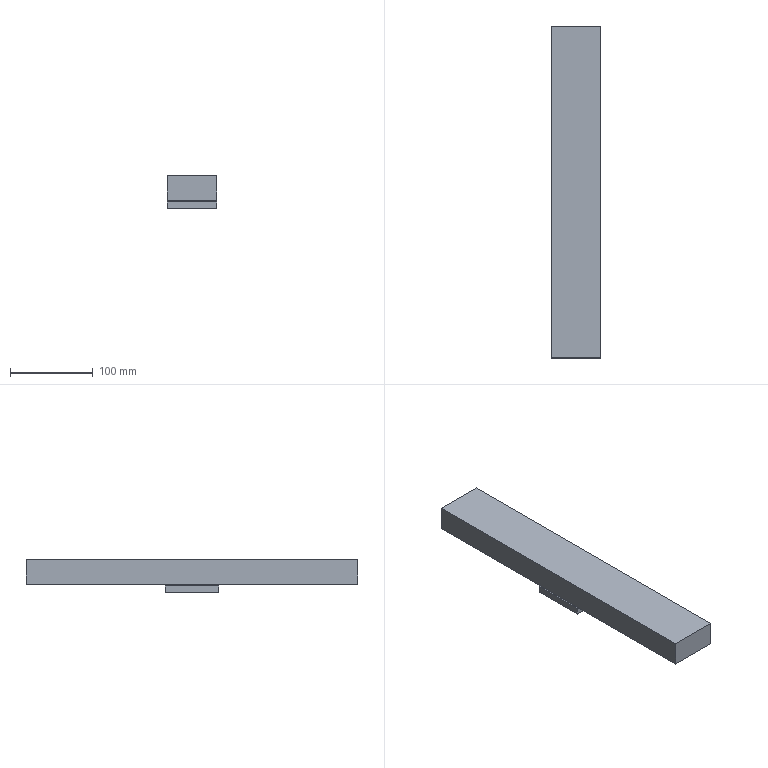Part | SolidWorks | features Cut 2, ICE 2, Chamfer 1, Extrusion 1, HoleWzd 1 | 1 solid | 13 faces | box 60 x 400 x 40 mm | volume 758635 mm3 | plane 13
STEP:
#1=CARTESIAN_POINT('',(-60.,32.5,8.));
#2=VERTEX_POINT('',#1);
#3=CARTESIAN_POINT('',(0.,32.5,8.));
#4=VERTEX_POINT('',#3);
#5=CARTESIAN_POINT('',(60.,32.5,8.));
#6=DIRECTION('',(1.,0.,0.));
#7=VECTOR('',#6,1000.);
#8=LINE('',#5,#7);
#9=EDGE_CURVE('',#2,#4,#8,.T.);
#10=ORIENTED_EDGE('',*,*,#9,.T.);
#11=CARTESIAN_POINT('',(0.,32.5,0.));
#12=VERTEX_POINT('',#11);
#13=CARTESIAN_POINT('',(0.,32.5,-88.459));
#14=DIRECTION('',(0.,0.,1.));
#15=VECTOR('',#14,1000.);
#16=LINE('',#13,#15);
#17=EDGE_CURVE('',#12,#4,#16,.T.);
#18=ORIENTED_EDGE('',*,*,#17,.F.);
#19=CARTESIAN_POINT('',(-60.,32.5,0.));
#20=VERTEX_POINT('',#19);
#21=CARTESIAN_POINT('',(-60.,32.5,0.));
#22=DIRECTION('',(-1.,0.,0.));
#23=VECTOR('',#22,1000.);
#24=LINE('',#21,#23);
#25=EDGE_CURVE('',#12,#20,#24,.T.);
#26=ORIENTED_EDGE('',*,*,#25,.T.);
#27=CARTESIAN_POINT('',(-60.,32.5,10.));
#28=DIRECTION('',(0.,0.,-1.));
#29=VECTOR('',#28,1000.);
#30=LINE('',#27,#29);
#31=EDGE_CURVE('',#2,#20,#30,.T.);
#32=ORIENTED_EDGE('',*,*,#31,.F.);
#33=EDGE_LOOP('',(#10,#18,#26,#32));
#34=FACE_OUTER_BOUND('',#33,.T.);
#35=CARTESIAN_POINT('',(-60.,32.5,10.));
#36=DIRECTION('',(0.,-1.,0.));
#37=DIRECTION('',(0.,0.,-1.));
#38=AXIS2_PLACEMENT_3D('',#35,#36,#37);
#39=PLANE('',#38);
#40=ADVANCED_FACE('',(#34),#39,.F.);
#41=CARTESIAN_POINT('',(-60.,-32.5,8.));
#42=VERTEX_POINT('',#41);
#43=CARTESIAN_POINT('',(-60.,-32.5,0.));
#44=VERTEX_POINT('',#43);
#45=CARTESIAN_POINT('',(-60.,-32.5,10.));
#46=DIRECTION('',(0.,0.,-1.));
#47=VECTOR('',#46,1000.);
#48=LINE('',#45,#47);
#49=EDGE_CURVE('',#42,#44,#48,.T.);
#50=ORIENTED_EDGE('',*,*,#49,.F.);
#51=CARTESIAN_POINT('',(-60.,32.5,8.));
#52=DIRECTION('',(0.,1.,0.));
#53=VECTOR('',#52,1000.);
#54=LINE('',#51,#53);
#55=EDGE_CURVE('',#42,#2,#54,.T.);
#56=ORIENTED_EDGE('',*,*,#55,.T.);
#57=ORIENTED_EDGE('',*,*,#31,.T.);
#58=CARTESIAN_POINT('',(-60.,32.5,0.));
#59=DIRECTION('',(0.,-1.,0.));
#60=VECTOR('',#59,1000.);
#61=LINE('',#58,#60);
#62=EDGE_CURVE('',#20,#44,#61,.T.);
#63=ORIENTED_EDGE('',*,*,#62,.T.);
#64=EDGE_LOOP('',(#50,#56,#57,#63));
#65=FACE_OUTER_BOUND('',#64,.T.);
#66=CARTESIAN_POINT('',(-60.,32.5,10.));
#67=DIRECTION('',(1.,0.,0.));
#68=DIRECTION('',(0.,1.,0.));
#69=AXIS2_PLACEMENT_3D('',#66,#67,#68);
#70=PLANE('',#69);
#71=ADVANCED_FACE('',(#65),#70,.F.);
#72=CARTESIAN_POINT('',(0.,-32.5,0.));
#73=VERTEX_POINT('',#72);
#74=CARTESIAN_POINT('',(-60.,-32.5,0.));
#75=DIRECTION('',(1.,0.,0.));
#76=VECTOR('',#75,1000.);
#77=LINE('',#74,#76);
#78=EDGE_CURVE('',#44,#73,#77,.T.);
#79=ORIENTED_EDGE('',*,*,#78,.T.);
#80=CARTESIAN_POINT('',(0.,-32.5,8.));
#81=VERTEX_POINT('',#80);
#82=CARTESIAN_POINT('',(0.,-32.5,-88.459));
#83=DIRECTION('',(0.,0.,1.));
#84=VECTOR('',#83,1000.);
#85=LINE('',#82,#84);
#86=EDGE_CURVE('',#73,#81,#85,.T.);
#87=ORIENTED_EDGE('',*,*,#86,.T.);
#88=CARTESIAN_POINT('',(-60.,-32.5,8.));
#89=DIRECTION('',(-1.,0.,0.));
#90=VECTOR('',#89,1000.);
#91=LINE('',#88,#90);
#92=EDGE_CURVE('',#81,#42,#91,.T.);
#93=ORIENTED_EDGE('',*,*,#92,.T.);
#94=ORIENTED_EDGE('',*,*,#49,.T.);
#95=EDGE_LOOP('',(#79,#87,#93,#94));
#96=FACE_OUTER_BOUND('',#95,.T.);
#97=CARTESIAN_POINT('',(-60.,-32.5,10.));
#98=DIRECTION('',(0.,1.,0.));
#99=DIRECTION('',(0.,0.,1.));
#100=AXIS2_PLACEMENT_3D('',#97,#98,#99);
#101=PLANE('',#100);
#102=ADVANCED_FACE('',(#96),#101,.F.);
#103=ORIENTED_EDGE('',*,*,#25,.F.);
#104=CARTESIAN_POINT('',(0.,32.5,0.));
#105=DIRECTION('',(0.,1.,0.));
#106=VECTOR('',#105,1000.);
#107=LINE('',#104,#106);
#108=EDGE_CURVE('',#73,#12,#107,.T.);
#109=ORIENTED_EDGE('',*,*,#108,.F.);
#110=ORIENTED_EDGE('',*,*,#78,.F.);
#111=ORIENTED_EDGE('',*,*,#62,.F.);
#112=EDGE_LOOP('',(#103,#109,#110,#111));
#113=FACE_OUTER_BOUND('',#112,.T.);
#114=CARTESIAN_POINT('',(0.,0.,0.));
#115=DIRECTION('',(0.,0.,1.));
#116=DIRECTION('',(1.,0.,0.));
#117=AXIS2_PLACEMENT_3D('',#114,#115,#116);
#118=PLANE('',#117);
#119=ADVANCED_FACE('',(#113),#118,.F.);
#120=CARTESIAN_POINT('',(-58.,30.5,10.));
#121=VERTEX_POINT('',#120);
#122=CARTESIAN_POINT('',(-38.667,11.167,29.333));
#123=DIRECTION('',(0.5774,-0.5774,0.5774));
#124=VECTOR('',#123,1000.);
#125=LINE('',#122,#124);
#126=EDGE_CURVE('',#2,#121,#125,.T.);
#127=ORIENTED_EDGE('',*,*,#126,.F.);
#128=ORIENTED_EDGE('',*,*,#55,.F.);
#129=CARTESIAN_POINT('',(-58.,-30.5,10.));
#130=VERTEX_POINT('',#129);
#131=CARTESIAN_POINT('',(-47.833,-20.333,20.167));
#132=DIRECTION('',(-0.5774,-0.5774,-0.5774));
#133=VECTOR('',#132,1000.);
#134=LINE('',#131,#133);
#135=EDGE_CURVE('',#130,#42,#134,.T.);
#136=ORIENTED_EDGE('',*,*,#135,.F.);
#137=CARTESIAN_POINT('',(-58.,-32.5,10.));
#138=DIRECTION('',(0.,-1.,0.));
#139=VECTOR('',#138,1000.);
#140=LINE('',#137,#139);
#141=EDGE_CURVE('',#121,#130,#140,.T.);
#142=ORIENTED_EDGE('',*,*,#141,.F.);
#143=EDGE_LOOP('',(#127,#128,#136,#142));
#144=FACE_OUTER_BOUND('',#143,.T.);
#145=CARTESIAN_POINT('',(-58.,0.,10.));
#146=DIRECTION('',(-0.7071,0.,0.7071));
#147=DIRECTION('',(0.,1.,0.));
#148=AXIS2_PLACEMENT_3D('',#145,#146,#147);
#149=PLANE('',#148);
#150=ADVANCED_FACE('',(#144),#149,.T.);
#151=CARTESIAN_POINT('',(0.,-30.5,10.));
#152=VERTEX_POINT('',#151);
#153=CARTESIAN_POINT('',(0.,-30.5,10.));
#154=DIRECTION('',(0.,-0.7071,-0.7071));
#155=VECTOR('',#154,1000.);
#156=LINE('',#153,#155);
#157=EDGE_CURVE('',#152,#81,#156,.T.);
#158=ORIENTED_EDGE('',*,*,#157,.F.);
#159=CARTESIAN_POINT('',(60.,-30.5,10.));
#160=DIRECTION('',(1.,0.,0.));
#161=VECTOR('',#160,1000.);
#162=LINE('',#159,#161);
#163=EDGE_CURVE('',#130,#152,#162,.T.);
#164=ORIENTED_EDGE('',*,*,#163,.F.);
#165=ORIENTED_EDGE('',*,*,#135,.T.);
#166=ORIENTED_EDGE('',*,*,#92,.F.);
#167=EDGE_LOOP('',(#158,#164,#165,#166));
#168=FACE_OUTER_BOUND('',#167,.T.);
#169=CARTESIAN_POINT('',(0.,-30.5,10.));
#170=DIRECTION('',(0.,-0.7071,0.7071));
#171=DIRECTION('',(-1.,0.,0.));
#172=AXIS2_PLACEMENT_3D('',#169,#170,#171);
#173=PLANE('',#172);
#174=ADVANCED_FACE('',(#168),#173,.T.);
#175=CARTESIAN_POINT('',(0.,30.5,10.));
#176=VERTEX_POINT('',#175);
#177=CARTESIAN_POINT('',(0.,30.5,10.));
#178=DIRECTION('',(0.,-0.7071,0.7071));
#179=VECTOR('',#178,1000.);
#180=LINE('',#177,#179);
#181=EDGE_CURVE('',#4,#176,#180,.T.);
#182=ORIENTED_EDGE('',*,*,#181,.F.);
#183=ORIENTED_EDGE('',*,*,#9,.F.);
#184=ORIENTED_EDGE('',*,*,#126,.T.);
#185=CARTESIAN_POINT('',(-60.,30.5,10.));
#186=DIRECTION('',(-1.,0.,0.));
#187=VECTOR('',#186,1000.);
#188=LINE('',#185,#187);
#189=EDGE_CURVE('',#176,#121,#188,.T.);
#190=ORIENTED_EDGE('',*,*,#189,.F.);
#191=EDGE_LOOP('',(#182,#183,#184,#190));
#192=FACE_OUTER_BOUND('',#191,.T.);
#193=CARTESIAN_POINT('',(0.,30.5,10.));
#194=DIRECTION('',(0.,0.7071,0.7071));
#195=DIRECTION('',(1.,0.,0.));
#196=AXIS2_PLACEMENT_3D('',#193,#194,#195);
#197=PLANE('',#196);
#198=ADVANCED_FACE('',(#192),#197,.T.);
#199=CARTESIAN_POINT('',(0.,200.,10.));
#200=VERTEX_POINT('',#199);
#201=CARTESIAN_POINT('',(0.,200.,10.));
#202=DIRECTION('',(0.,-1.,0.));
#203=VECTOR('',#202,1000.);
#204=LINE('',#201,#203);
#205=EDGE_CURVE('',#200,#176,#204,.T.);
#206=ORIENTED_EDGE('',*,*,#205,.T.);
#207=ORIENTED_EDGE('',*,*,#189,.T.);
#208=ORIENTED_EDGE('',*,*,#141,.T.);
#209=ORIENTED_EDGE('',*,*,#163,.T.);
#210=CARTESIAN_POINT('',(0.,-200.,10.));
#211=VERTEX_POINT('',#210);
#212=CARTESIAN_POINT('',(0.,200.,10.));
#213=DIRECTION('',(0.,-1.,0.));
#214=VECTOR('',#213,1000.);
#215=LINE('',#212,#214);
#216=EDGE_CURVE('',#152,#211,#215,.T.);
#217=ORIENTED_EDGE('',*,*,#216,.T.);
#218=CARTESIAN_POINT('',(-60.,-200.,10.));
#219=VERTEX_POINT('',#218);
#220=CARTESIAN_POINT('',(0.,-200.,10.));
#221=DIRECTION('',(-1.,0.,0.));
#222=VECTOR('',#221,1000.);
#223=LINE('',#220,#222);
#224=EDGE_CURVE('',#211,#219,#223,.T.);
#225=ORIENTED_EDGE('',*,*,#224,.T.);
#226=CARTESIAN_POINT('',(-60.,200.,10.));
#227=VERTEX_POINT('',#226);
#228=CARTESIAN_POINT('',(-60.,32.5,10.));
#229=DIRECTION('',(0.,-1.,0.));
#230=VECTOR('',#229,1000.);
#231=LINE('',#228,#230);
#232=EDGE_CURVE('',#227,#219,#231,.T.);
#233=ORIENTED_EDGE('',*,*,#232,.F.);
#234=CARTESIAN_POINT('',(0.,200.,10.));
#235=DIRECTION('',(1.,0.,0.));
#236=VECTOR('',#235,1000.);
#237=LINE('',#234,#236);
#238=EDGE_CURVE('',#227,#200,#237,.T.);
#239=ORIENTED_EDGE('',*,*,#238,.T.);
#240=EDGE_LOOP('',(#206,#207,#208,#209,#217,#225,#233,#239));
#241=FACE_OUTER_BOUND('',#240,.T.);
#242=CARTESIAN_POINT('',(0.,0.,10.));
#243=DIRECTION('',(0.,0.,1.));
#244=DIRECTION('',(1.,0.,0.));
#245=AXIS2_PLACEMENT_3D('',#242,#243,#244);
#246=PLANE('',#245);
#247=ADVANCED_FACE('',(#241),#246,.F.);
#248=ORIENTED_EDGE('',*,*,#232,.T.);
#249=CARTESIAN_POINT('',(-60.,-200.,40.));
#250=VERTEX_POINT('',#249);
#251=CARTESIAN_POINT('',(-60.,-200.,-394.475));
#252=DIRECTION('',(0.,0.,1.));
#253=VECTOR('',#252,1000.);
#254=LINE('',#251,#253);
#255=EDGE_CURVE('',#219,#250,#254,.T.);
#256=ORIENTED_EDGE('',*,*,#255,.T.);
#257=CARTESIAN_POINT('',(-60.,200.,40.));
#258=VERTEX_POINT('',#257);
#259=CARTESIAN_POINT('',(-60.,32.5,40.));
#260=DIRECTION('',(0.,-1.,0.));
#261=VECTOR('',#260,1000.);
#262=LINE('',#259,#261);
#263=EDGE_CURVE('',#258,#250,#262,.T.);
#264=ORIENTED_EDGE('',*,*,#263,.F.);
#265=CARTESIAN_POINT('',(-60.,200.,-394.475));
#266=DIRECTION('',(0.,0.,1.));
#267=VECTOR('',#266,1000.);
#268=LINE('',#265,#267);
#269=EDGE_CURVE('',#227,#258,#268,.T.);
#270=ORIENTED_EDGE('',*,*,#269,.F.);
#271=EDGE_LOOP('',(#248,#256,#264,#270));
#272=FACE_OUTER_BOUND('',#271,.T.);
#273=CARTESIAN_POINT('',(-60.,32.5,40.));
#274=DIRECTION('',(1.,0.,0.));
#275=DIRECTION('',(0.,0.,-1.));
#276=AXIS2_PLACEMENT_3D('',#273,#274,#275);
#277=PLANE('',#276);
#278=ADVANCED_FACE('',(#272),#277,.F.);
#279=CARTESIAN_POINT('',(0.,-200.,40.));
#280=VERTEX_POINT('',#279);
#281=CARTESIAN_POINT('',(0.,-200.,40.));
#282=DIRECTION('',(1.,0.,0.));
#283=VECTOR('',#282,1000.);
#284=LINE('',#281,#283);
#285=EDGE_CURVE('',#250,#280,#284,.T.);
#286=ORIENTED_EDGE('',*,*,#285,.T.);
#287=CARTESIAN_POINT('',(0.,200.,40.));
#288=VERTEX_POINT('',#287);
#289=CARTESIAN_POINT('',(0.,200.,40.));
#290=DIRECTION('',(0.,1.,0.));
#291=VECTOR('',#290,1000.);
#292=LINE('',#289,#291);
#293=EDGE_CURVE('',#280,#288,#292,.T.);
#294=ORIENTED_EDGE('',*,*,#293,.T.);
#295=CARTESIAN_POINT('',(0.,200.,40.));
#296=DIRECTION('',(-1.,0.,0.));
#297=VECTOR('',#296,1000.);
#298=LINE('',#295,#297);
#299=EDGE_CURVE('',#288,#258,#298,.T.);
#300=ORIENTED_EDGE('',*,*,#299,.T.);
#301=ORIENTED_EDGE('',*,*,#263,.T.);
#302=EDGE_LOOP('',(#286,#294,#300,#301));
#303=FACE_OUTER_BOUND('',#302,.T.);
#304=CARTESIAN_POINT('',(0.,0.,40.));
#305=DIRECTION('',(0.,0.,1.));
#306=DIRECTION('',(1.,0.,0.));
#307=AXIS2_PLACEMENT_3D('',#304,#305,#306);
#308=PLANE('',#307);
#309=ADVANCED_FACE('',(#303),#308,.T.);
#310=ORIENTED_EDGE('',*,*,#224,.F.);
#311=CARTESIAN_POINT('',(0.,-200.,-394.475));
#312=DIRECTION('',(0.,0.,1.));
#313=VECTOR('',#312,1000.);
#314=LINE('',#311,#313);
#315=EDGE_CURVE('',#211,#280,#314,.T.);
#316=ORIENTED_EDGE('',*,*,#315,.T.);
#317=ORIENTED_EDGE('',*,*,#285,.F.);
#318=ORIENTED_EDGE('',*,*,#255,.F.);
#319=EDGE_LOOP('',(#310,#316,#317,#318));
#320=FACE_OUTER_BOUND('',#319,.T.);
#321=CARTESIAN_POINT('',(0.,-200.,-394.475));
#322=DIRECTION('',(0.,-1.,0.));
#323=DIRECTION('',(0.,0.,-1.));
#324=AXIS2_PLACEMENT_3D('',#321,#322,#323);
#325=PLANE('',#324);
#326=ADVANCED_FACE('',(#320),#325,.T.);
#327=ORIENTED_EDGE('',*,*,#293,.F.);
#328=ORIENTED_EDGE('',*,*,#315,.F.);
#329=ORIENTED_EDGE('',*,*,#216,.F.);
#330=ORIENTED_EDGE('',*,*,#157,.T.);
#331=ORIENTED_EDGE('',*,*,#86,.F.);
#332=ORIENTED_EDGE('',*,*,#108,.T.);
#333=ORIENTED_EDGE('',*,*,#17,.T.);
#334=ORIENTED_EDGE('',*,*,#181,.T.);
#335=ORIENTED_EDGE('',*,*,#205,.F.);
#336=CARTESIAN_POINT('',(0.,200.,-394.475));
#337=DIRECTION('',(0.,0.,1.));
#338=VECTOR('',#337,1000.);
#339=LINE('',#336,#338);
#340=EDGE_CURVE('',#200,#288,#339,.T.);
#341=ORIENTED_EDGE('',*,*,#340,.T.);
#342=EDGE_LOOP('',(#327,#328,#329,#330,#331,#332,#333,#334,#335,#341));
#343=FACE_OUTER_BOUND('',#342,.T.);
#344=CARTESIAN_POINT('',(0.,200.,-394.475));
#345=DIRECTION('',(1.,0.,0.));
#346=DIRECTION('',(0.,1.,0.));
#347=AXIS2_PLACEMENT_3D('',#344,#345,#346);
#348=PLANE('',#347);
#349=ADVANCED_FACE('',(#343),#348,.T.);
#350=ORIENTED_EDGE('',*,*,#238,.F.);
#351=ORIENTED_EDGE('',*,*,#269,.T.);
#352=ORIENTED_EDGE('',*,*,#299,.F.);
#353=ORIENTED_EDGE('',*,*,#340,.F.);
#354=EDGE_LOOP('',(#350,#351,#352,#353));
#355=FACE_OUTER_BOUND('',#354,.T.);
#356=CARTESIAN_POINT('',(0.,200.,-394.475));
#357=DIRECTION('',(0.,1.,0.));
#358=DIRECTION('',(0.,0.,1.));
#359=AXIS2_PLACEMENT_3D('',#356,#357,#358);
#360=PLANE('',#359);
#361=ADVANCED_FACE('',(#355),#360,.T.);
#362=CLOSED_SHELL('',(#40,#71,#102,#119,#150,#174,#198,#247,#278,#309,#326,#349,#361));
#363=MANIFOLD_SOLID_BREP('',#362);
#364=CARTESIAN_POINT('',(0.,0.,0.));
#365=DIRECTION('',(0.,0.,1.));
#366=DIRECTION('',(1.,0.,0.));
#367=AXIS2_PLACEMENT_3D('',#364,#365,#366);
#368=(LENGTH_UNIT()NAMED_UNIT(*)SI_UNIT(.MILLI.,.METRE.));
#369=UNCERTAINTY_MEASURE_WITH_UNIT(LENGTH_MEASURE(0.00001),#368,'','');
#370=(NAMED_UNIT(*)PLANE_ANGLE_UNIT()SI_UNIT($,.RADIAN.));
#371=(NAMED_UNIT(*)SI_UNIT($,.STERADIAN.)SOLID_ANGLE_UNIT());
#372=(GEOMETRIC_REPRESENTATION_CONTEXT(3)GLOBAL_UNCERTAINTY_ASSIGNED_CONTEXT((#369))GLOBAL_UNIT_ASSIGNED_CONTEXT((#368,#370,#371))REPRESENTATION_CONTEXT('',''));
#373=ADVANCED_BREP_SHAPE_REPRESENTATION('',(#363,#367),#372);